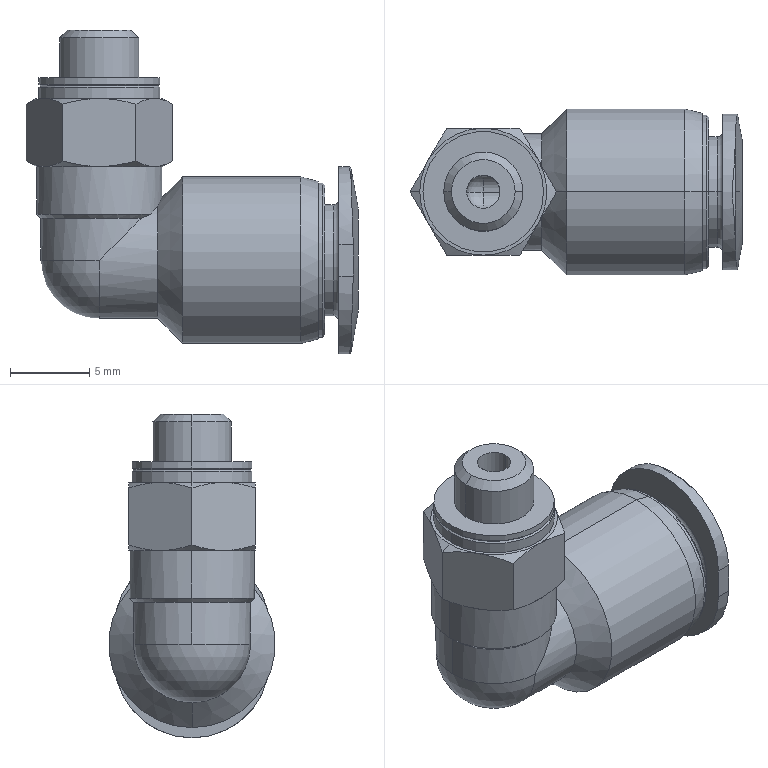Part | SolidWorks | features RefAxis 9, 3DProfileFeature 3, Revolution 3, ICE 2, RevCut 2 | 1 solid | 82 faces | box 20.919 x 10.5 x 20.4 mm | volume 1362 mm3 | cone 29 | cylinder 27 | plane 16 | torus 7 | sphere 3 | commonest cylinder face diameters 2.1 x4 7.35 x4 7.6 x4 9.8 x3 5 x2 6 x2